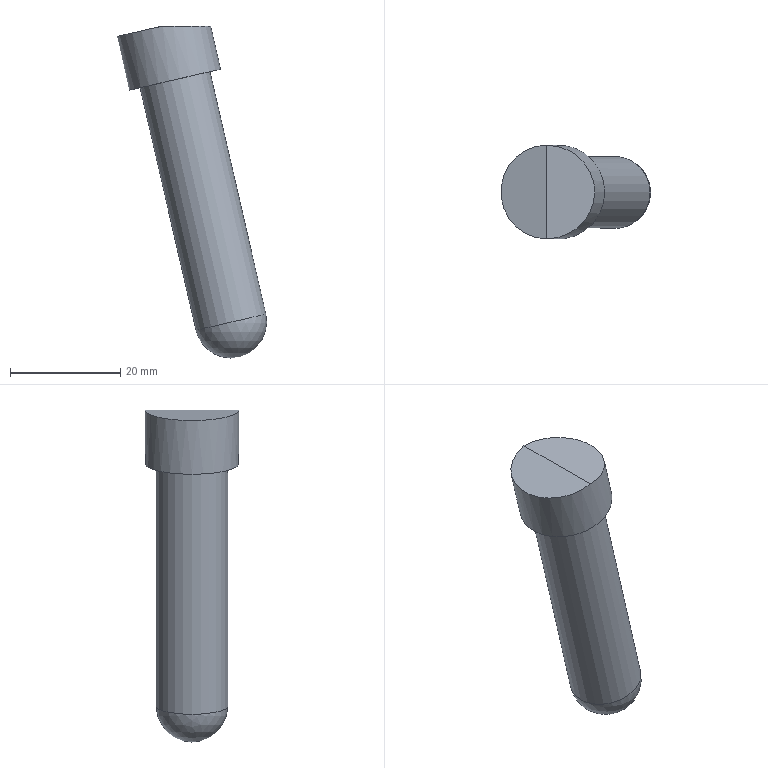Part | STEP file | solid 4 | 1 solid | 6 faces | box 27.19 x 17 x 60.243 mm | volume 8744 mm3 | plane 3 | cylinder 2 | sphere 1 | commonest cylinder face diameters 13 x1 17 x1